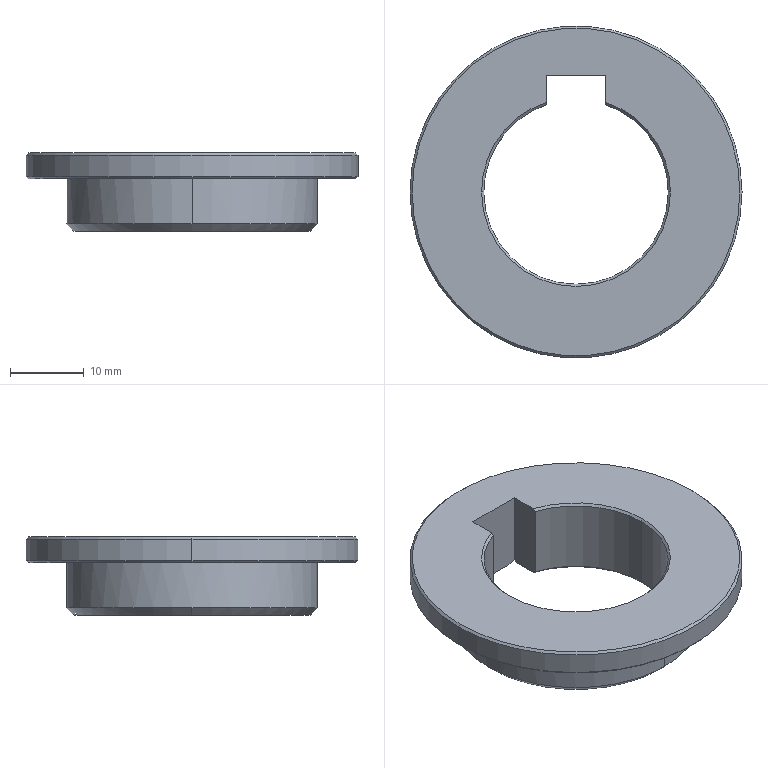Part | NX | 1 solid | 26 faces | box 45 x 45 x 10.6 mm | volume 6440 mm3 | cone 12 | plane 7 | cylinder 7 | commonest cylinder face diameters 25 x3 34 x2 45 x2
STEP:
#1=CARTESIAN_POINT('',(22.2,0.,-3.5));
#2=VERTEX_POINT('',#1);
#3=CARTESIAN_POINT('',(-22.2,0.,-3.5));
#4=VERTEX_POINT('',#3);
#5=CARTESIAN_POINT('',(0.,0.,-3.5));
#6=DIRECTION('',(0.,0.,1.));
#7=DIRECTION('',(1.,0.,0.));
#8=AXIS2_PLACEMENT_3D('',#5,#6,#7);
#9=CIRCLE('',#8,22.2);
#10=EDGE_CURVE('',#2,#4,#9,.T.);
#11=ORIENTED_EDGE('',*,*,#10,.F.);
#12=CARTESIAN_POINT('',(0.,0.,-3.5));
#13=DIRECTION('',(0.,0.,1.));
#14=DIRECTION('',(1.,0.,0.));
#15=AXIS2_PLACEMENT_3D('',#12,#13,#14);
#16=CIRCLE('',#15,22.2);
#17=EDGE_CURVE('',#4,#2,#16,.T.);
#18=ORIENTED_EDGE('',*,*,#17,.F.);
#19=EDGE_LOOP('',(#11,#18));
#20=FACE_BOUND('',#19,.T.);
#21=CARTESIAN_POINT('',(0.,-17.,-3.5));
#22=VERTEX_POINT('',#21);
#23=CARTESIAN_POINT('',(0.,17.,-3.5));
#24=VERTEX_POINT('',#23);
#25=CARTESIAN_POINT('',(0.,0.,-3.5));
#26=DIRECTION('',(0.,0.,1.));
#27=DIRECTION('',(0.,1.,0.));
#28=AXIS2_PLACEMENT_3D('',#25,#26,#27);
#29=CIRCLE('',#28,17.);
#30=EDGE_CURVE('',#22,#24,#29,.T.);
#31=ORIENTED_EDGE('',*,*,#30,.T.);
#32=CARTESIAN_POINT('',(0.,0.,-3.5));
#33=DIRECTION('',(0.,0.,1.));
#34=DIRECTION('',(0.,1.,0.));
#35=AXIS2_PLACEMENT_3D('',#32,#33,#34);
#36=CIRCLE('',#35,17.);
#37=EDGE_CURVE('',#24,#22,#36,.T.);
#38=ORIENTED_EDGE('',*,*,#37,.T.);
#39=EDGE_LOOP('',(#31,#38));
#40=FACE_BOUND('',#39,.T.);
#41=CARTESIAN_POINT('',(0.,0.,-3.5));
#42=DIRECTION('',(0.,0.,1.));
#43=DIRECTION('',(1.,0.,0.));
#44=AXIS2_PLACEMENT_3D('',#41,#42,#43);
#45=PLANE('',#44);
#46=ADVANCED_FACE('',(#20,#40),#45,.F.);
#47=CARTESIAN_POINT('',(22.5,0.,-3.2));
#48=VERTEX_POINT('',#47);
#49=CARTESIAN_POINT('',(-22.5,0.,-3.2));
#50=VERTEX_POINT('',#49);
#51=CARTESIAN_POINT('',(0.,0.,-3.2));
#52=DIRECTION('',(0.,0.,1.));
#53=DIRECTION('',(1.,0.,0.));
#54=AXIS2_PLACEMENT_3D('',#51,#52,#53);
#55=CIRCLE('',#54,22.5);
#56=EDGE_CURVE('',#48,#50,#55,.T.);
#57=ORIENTED_EDGE('',*,*,#56,.T.);
#58=CARTESIAN_POINT('',(-22.5,0.,-0.3));
#59=VERTEX_POINT('',#58);
#60=CARTESIAN_POINT('',(-22.5,0.,0.));
#61=DIRECTION('',(0.,0.,-1.));
#62=VECTOR('',#61,1000.);
#63=LINE('',#60,#62);
#64=EDGE_CURVE('',#50,#59,#63,.F.);
#65=ORIENTED_EDGE('',*,*,#64,.T.);
#66=CARTESIAN_POINT('',(22.5,0.,-0.3));
#67=VERTEX_POINT('',#66);
#68=CARTESIAN_POINT('',(0.,0.,-0.3));
#69=DIRECTION('',(0.,0.,-1.));
#70=DIRECTION('',(-1.,0.,0.));
#71=AXIS2_PLACEMENT_3D('',#68,#69,#70);
#72=CIRCLE('',#71,22.5);
#73=EDGE_CURVE('',#59,#67,#72,.T.);
#74=ORIENTED_EDGE('',*,*,#73,.T.);
#75=CARTESIAN_POINT('',(22.5,0.,0.));
#76=DIRECTION('',(0.,0.,-1.));
#77=VECTOR('',#76,1000.);
#78=LINE('',#75,#77);
#79=EDGE_CURVE('',#48,#67,#78,.F.);
#80=ORIENTED_EDGE('',*,*,#79,.F.);
#81=EDGE_LOOP('',(#57,#65,#74,#80));
#82=FACE_BOUND('',#81,.T.);
#83=CARTESIAN_POINT('',(0.,0.,0.));
#84=DIRECTION('',(0.,0.,-1.));
#85=DIRECTION('',(-1.,0.,0.));
#86=AXIS2_PLACEMENT_3D('',#83,#84,#85);
#87=CYLINDRICAL_SURFACE('',#86,22.5);
#88=ADVANCED_FACE('',(#82),#87,.T.);
#89=CARTESIAN_POINT('',(12.5,0.,-0.3));
#90=VERTEX_POINT('',#89);
#91=CARTESIAN_POINT('',(12.5,0.,-10.3));
#92=VERTEX_POINT('',#91);
#93=CARTESIAN_POINT('',(12.5,0.,0.));
#94=DIRECTION('',(0.,0.,-1.));
#95=VECTOR('',#94,1000.);
#96=LINE('',#93,#95);
#97=EDGE_CURVE('',#90,#92,#96,.T.);
#98=ORIENTED_EDGE('',*,*,#97,.F.);
#99=CARTESIAN_POINT('',(4.,11.843,-0.3));
#100=VERTEX_POINT('',#99);
#101=CARTESIAN_POINT('',(0.,0.,-0.3));
#102=DIRECTION('',(0.,0.,1.));
#103=DIRECTION('',(1.,0.,0.));
#104=AXIS2_PLACEMENT_3D('',#101,#102,#103);
#105=CIRCLE('',#104,12.5);
#106=EDGE_CURVE('',#90,#100,#105,.T.);
#107=ORIENTED_EDGE('',*,*,#106,.T.);
#108=CARTESIAN_POINT('',(4.,11.843,-10.3));
#109=VERTEX_POINT('',#108);
#110=CARTESIAN_POINT('',(4.,11.843,0.));
#111=DIRECTION('',(0.,0.,-1.));
#112=VECTOR('',#111,1000.);
#113=LINE('',#110,#112);
#114=EDGE_CURVE('',#100,#109,#113,.T.);
#115=ORIENTED_EDGE('',*,*,#114,.T.);
#116=CARTESIAN_POINT('',(0.,0.,-10.3));
#117=DIRECTION('',(0.,0.,-1.));
#118=DIRECTION('',(-1.,0.,0.));
#119=AXIS2_PLACEMENT_3D('',#116,#117,#118);
#120=CIRCLE('',#119,12.5);
#121=EDGE_CURVE('',#109,#92,#120,.T.);
#122=ORIENTED_EDGE('',*,*,#121,.T.);
#123=EDGE_LOOP('',(#98,#107,#115,#122));
#124=FACE_BOUND('',#123,.T.);
#125=CARTESIAN_POINT('',(0.,0.,0.));
#126=DIRECTION('',(0.,0.,-1.));
#127=DIRECTION('',(-1.,0.,0.));
#128=AXIS2_PLACEMENT_3D('',#125,#126,#127);
#129=CYLINDRICAL_SURFACE('',#128,12.5);
#130=ADVANCED_FACE('',(#124),#129,.F.);
#131=CARTESIAN_POINT('',(22.2,0.,0.));
#132=VERTEX_POINT('',#131);
#133=CARTESIAN_POINT('',(-22.2,0.,0.));
#134=VERTEX_POINT('',#133);
#135=CARTESIAN_POINT('',(0.,0.,0.));
#136=DIRECTION('',(0.,0.,-1.));
#137=DIRECTION('',(-1.,0.,0.));
#138=AXIS2_PLACEMENT_3D('',#135,#136,#137);
#139=CIRCLE('',#138,22.2);
#140=EDGE_CURVE('',#132,#134,#139,.T.);
#141=ORIENTED_EDGE('',*,*,#140,.F.);
#142=CARTESIAN_POINT('',(0.,0.,0.));
#143=DIRECTION('',(0.,0.,-1.));
#144=DIRECTION('',(-1.,0.,0.));
#145=AXIS2_PLACEMENT_3D('',#142,#143,#144);
#146=CIRCLE('',#145,22.2);
#147=EDGE_CURVE('',#134,#132,#146,.T.);
#148=ORIENTED_EDGE('',*,*,#147,.F.);
#149=EDGE_LOOP('',(#141,#148));
#150=FACE_BOUND('',#149,.T.);
#151=CARTESIAN_POINT('',(-4.,12.159,0.));
#152=VERTEX_POINT('',#151);
#153=CARTESIAN_POINT('',(-12.8,0.,0.));
#154=VERTEX_POINT('',#153);
#155=CARTESIAN_POINT('',(0.,0.,0.));
#156=DIRECTION('',(0.,0.,1.));
#157=DIRECTION('',(1.,0.,0.));
#158=AXIS2_PLACEMENT_3D('',#155,#156,#157);
#159=CIRCLE('',#158,12.8);
#160=EDGE_CURVE('',#152,#154,#159,.T.);
#161=ORIENTED_EDGE('',*,*,#160,.F.);
#162=CARTESIAN_POINT('',(-4.,15.8,0.));
#163=VERTEX_POINT('',#162);
#164=CARTESIAN_POINT('',(-4.,0.,0.));
#165=DIRECTION('',(0.,-1.,0.));
#166=VECTOR('',#165,1000.);
#167=LINE('',#164,#166);
#168=EDGE_CURVE('',#163,#152,#167,.T.);
#169=ORIENTED_EDGE('',*,*,#168,.F.);
#170=CARTESIAN_POINT('',(4.,15.8,0.));
#171=VERTEX_POINT('',#170);
#172=CARTESIAN_POINT('',(0.,15.8,0.));
#173=DIRECTION('',(-1.,0.,0.));
#174=VECTOR('',#173,1000.);
#175=LINE('',#172,#174);
#176=EDGE_CURVE('',#171,#163,#175,.T.);
#177=ORIENTED_EDGE('',*,*,#176,.F.);
#178=CARTESIAN_POINT('',(4.,12.159,0.));
#179=VERTEX_POINT('',#178);
#180=CARTESIAN_POINT('',(4.,0.,0.));
#181=DIRECTION('',(0.,1.,0.));
#182=VECTOR('',#181,1000.);
#183=LINE('',#180,#182);
#184=EDGE_CURVE('',#179,#171,#183,.T.);
#185=ORIENTED_EDGE('',*,*,#184,.F.);
#186=CARTESIAN_POINT('',(12.8,0.,0.));
#187=VERTEX_POINT('',#186);
#188=CARTESIAN_POINT('',(0.,0.,0.));
#189=DIRECTION('',(0.,0.,1.));
#190=DIRECTION('',(1.,0.,0.));
#191=AXIS2_PLACEMENT_3D('',#188,#189,#190);
#192=CIRCLE('',#191,12.8);
#193=EDGE_CURVE('',#187,#179,#192,.T.);
#194=ORIENTED_EDGE('',*,*,#193,.F.);
#195=CARTESIAN_POINT('',(0.,0.,0.));
#196=DIRECTION('',(0.,0.,1.));
#197=DIRECTION('',(1.,0.,0.));
#198=AXIS2_PLACEMENT_3D('',#195,#196,#197);
#199=CIRCLE('',#198,12.8);
#200=EDGE_CURVE('',#154,#187,#199,.T.);
#201=ORIENTED_EDGE('',*,*,#200,.F.);
#202=EDGE_LOOP('',(#161,#169,#177,#185,#194,#201));
#203=FACE_BOUND('',#202,.T.);
#204=CARTESIAN_POINT('',(0.,0.,0.));
#205=DIRECTION('',(0.,0.,1.));
#206=DIRECTION('',(1.,0.,0.));
#207=AXIS2_PLACEMENT_3D('',#204,#205,#206);
#208=PLANE('',#207);
#209=ADVANCED_FACE('',(#150,#203),#208,.T.);
#210=CARTESIAN_POINT('',(0.,17.,-9.6));
#211=VERTEX_POINT('',#210);
#212=CARTESIAN_POINT('',(17.,0.,-9.6));
#213=VERTEX_POINT('',#212);
#214=CARTESIAN_POINT('',(0.,0.,-9.6));
#215=DIRECTION('',(0.,0.,-1.));
#216=DIRECTION('',(1.,0.,0.));
#217=AXIS2_PLACEMENT_3D('',#214,#215,#216);
#218=CIRCLE('',#217,17.);
#219=EDGE_CURVE('',#211,#213,#218,.T.);
#220=ORIENTED_EDGE('',*,*,#219,.F.);
#221=CARTESIAN_POINT('',(0.,17.,-3.5));
#222=DIRECTION('',(0.,0.,-1.));
#223=VECTOR('',#222,1000.);
#224=LINE('',#221,#223);
#225=EDGE_CURVE('',#211,#24,#224,.F.);
#226=ORIENTED_EDGE('',*,*,#225,.T.);
#227=ORIENTED_EDGE('',*,*,#30,.F.);
#228=CARTESIAN_POINT('',(0.,-17.,-9.6));
#229=VERTEX_POINT('',#228);
#230=CARTESIAN_POINT('',(0.,-17.,-3.5));
#231=DIRECTION('',(0.,0.,-1.));
#232=VECTOR('',#231,1000.);
#233=LINE('',#230,#232);
#234=EDGE_CURVE('',#229,#22,#233,.F.);
#235=ORIENTED_EDGE('',*,*,#234,.F.);
#236=CARTESIAN_POINT('',(0.,0.,-9.6));
#237=DIRECTION('',(0.,0.,-1.));
#238=DIRECTION('',(1.,0.,0.));
#239=AXIS2_PLACEMENT_3D('',#236,#237,#238);
#240=CIRCLE('',#239,17.);
#241=EDGE_CURVE('',#213,#229,#240,.T.);
#242=ORIENTED_EDGE('',*,*,#241,.F.);
#243=EDGE_LOOP('',(#220,#226,#227,#235,#242));
#244=FACE_BOUND('',#243,.T.);
#245=CARTESIAN_POINT('',(0.,0.,-3.5));
#246=DIRECTION('',(0.,0.,-1.));
#247=DIRECTION('',(0.,1.,0.));
#248=AXIS2_PLACEMENT_3D('',#245,#246,#247);
#249=CYLINDRICAL_SURFACE('',#248,17.);
#250=ADVANCED_FACE('',(#244),#249,.T.);
#251=CARTESIAN_POINT('',(4.,12.159,-10.6));
#252=VERTEX_POINT('',#251);
#253=CARTESIAN_POINT('',(12.8,0.,-10.6));
#254=VERTEX_POINT('',#253);
#255=CARTESIAN_POINT('',(0.,0.,-10.6));
#256=DIRECTION('',(0.,0.,-1.));
#257=DIRECTION('',(-1.,0.,0.));
#258=AXIS2_PLACEMENT_3D('',#255,#256,#257);
#259=CIRCLE('',#258,12.8);
#260=EDGE_CURVE('',#252,#254,#259,.T.);
#261=ORIENTED_EDGE('',*,*,#260,.F.);
#262=CARTESIAN_POINT('',(4.,15.492,-10.6));
#263=VERTEX_POINT('',#262);
#264=CARTESIAN_POINT('',(4.,0.,-10.6));
#265=DIRECTION('',(0.,1.,0.));
#266=VECTOR('',#265,1000.);
#267=LINE('',#264,#266);
#268=EDGE_CURVE('',#252,#263,#267,.T.);
#269=ORIENTED_EDGE('',*,*,#268,.T.);
#270=CARTESIAN_POINT('',(16.,0.,-10.6));
#271=VERTEX_POINT('',#270);
#272=CARTESIAN_POINT('',(0.,0.,-10.6));
#273=DIRECTION('',(0.,0.,-1.));
#274=DIRECTION('',(1.,0.,0.));
#275=AXIS2_PLACEMENT_3D('',#272,#273,#274);
#276=CIRCLE('',#275,16.);
#277=EDGE_CURVE('',#263,#271,#276,.T.);
#278=ORIENTED_EDGE('',*,*,#277,.T.);
#279=CARTESIAN_POINT('',(-16.,0.,-10.6));
#280=VERTEX_POINT('',#279);
#281=CARTESIAN_POINT('',(0.,0.,-10.6));
#282=DIRECTION('',(0.,0.,-1.));
#283=DIRECTION('',(1.,0.,0.));
#284=AXIS2_PLACEMENT_3D('',#281,#282,#283);
#285=CIRCLE('',#284,16.);
#286=EDGE_CURVE('',#271,#280,#285,.T.);
#287=ORIENTED_EDGE('',*,*,#286,.T.);
#288=CARTESIAN_POINT('',(-4.,15.492,-10.6));
#289=VERTEX_POINT('',#288);
#290=CARTESIAN_POINT('',(0.,0.,-10.6));
#291=DIRECTION('',(0.,0.,-1.));
#292=DIRECTION('',(1.,0.,0.));
#293=AXIS2_PLACEMENT_3D('',#290,#291,#292);
#294=CIRCLE('',#293,16.);
#295=EDGE_CURVE('',#280,#289,#294,.T.);
#296=ORIENTED_EDGE('',*,*,#295,.T.);
#297=CARTESIAN_POINT('',(-4.,12.159,-10.6));
#298=VERTEX_POINT('',#297);
#299=CARTESIAN_POINT('',(-4.,0.,-10.6));
#300=DIRECTION('',(0.,-1.,0.));
#301=VECTOR('',#300,1000.);
#302=LINE('',#299,#301);
#303=EDGE_CURVE('',#289,#298,#302,.T.);
#304=ORIENTED_EDGE('',*,*,#303,.T.);
#305=CARTESIAN_POINT('',(-12.8,0.,-10.6));
#306=VERTEX_POINT('',#305);
#307=CARTESIAN_POINT('',(0.,0.,-10.6));
#308=DIRECTION('',(0.,0.,-1.));
#309=DIRECTION('',(-1.,0.,0.));
#310=AXIS2_PLACEMENT_3D('',#307,#308,#309);
#311=CIRCLE('',#310,12.8);
#312=EDGE_CURVE('',#306,#298,#311,.T.);
#313=ORIENTED_EDGE('',*,*,#312,.F.);
#314=CARTESIAN_POINT('',(0.,0.,-10.6));
#315=DIRECTION('',(0.,0.,-1.));
#316=DIRECTION('',(-1.,0.,0.));
#317=AXIS2_PLACEMENT_3D('',#314,#315,#316);
#318=CIRCLE('',#317,12.8);
#319=EDGE_CURVE('',#254,#306,#318,.T.);
#320=ORIENTED_EDGE('',*,*,#319,.F.);
#321=EDGE_LOOP('',(#261,#269,#278,#287,#296,#304,#313,#320));
#322=FACE_BOUND('',#321,.T.);
#323=CARTESIAN_POINT('',(-14.369,9.107,-10.6));
#324=DIRECTION('',(0.,0.,1.));
#325=DIRECTION('',(1.,0.,0.));
#326=AXIS2_PLACEMENT_3D('',#323,#324,#325);
#327=PLANE('',#326);
#328=ADVANCED_FACE('',(#322),#327,.F.);
#329=ORIENTED_EDGE('',*,*,#219,.T.);
#330=CARTESIAN_POINT('',(16.,0.,-10.6));
#331=DIRECTION('',(0.7071,0.,0.7071));
#332=VECTOR('',#331,1000.);
#333=LINE('',#330,#332);
#334=EDGE_CURVE('',#213,#271,#333,.F.);
#335=ORIENTED_EDGE('',*,*,#334,.T.);
#336=ORIENTED_EDGE('',*,*,#277,.F.);
#337=CARTESIAN_POINT('',(4.,15.8,-10.302));
#338=VERTEX_POINT('',#337);
#339=CARTESIAN_POINT('',(4.,15.492,-10.6));
#340=CARTESIAN_POINT('',(4.,15.518,-10.575));
#341=CARTESIAN_POINT('',(4.,15.543,-10.55));
#342=CARTESIAN_POINT('',(4.,15.569,-10.525));
#343=CARTESIAN_POINT('',(4.,15.595,-10.501));
#344=CARTESIAN_POINT('',(4.,15.62,-10.476));
#345=CARTESIAN_POINT('',(4.,15.646,-10.451));
#346=CARTESIAN_POINT('',(4.,15.672,-10.426));
#347=CARTESIAN_POINT('',(4.,15.697,-10.401));
#348=CARTESIAN_POINT('',(4.,15.723,-10.376));
#349=CARTESIAN_POINT('',(4.,15.749,-10.351));
#350=CARTESIAN_POINT('',(4.,15.774,-10.326));
#351=CARTESIAN_POINT('',(4.,15.8,-10.302));
#352=B_SPLINE_CURVE_WITH_KNOTS('',3,(#339,#340,#341,#342,#343,#344,#345,#346,#347,#348,#349,#350,#351),.UNSPECIFIED.,.F.,.F.,(4,3,3,3,4),(0.,0.1072,0.2145,0.3217,0.4289),.UNSPECIFIED.);
#353=EDGE_CURVE('',#263,#338,#352,.T.);
#354=ORIENTED_EDGE('',*,*,#353,.T.);
#355=CARTESIAN_POINT('',(2.522,15.8,-10.6));
#356=VERTEX_POINT('',#355);
#357=CARTESIAN_POINT('',(4.,15.8,-10.302));
#358=CARTESIAN_POINT('',(3.878,15.8,-10.331));
#359=CARTESIAN_POINT('',(3.756,15.8,-10.36));
#360=CARTESIAN_POINT('',(3.634,15.8,-10.388));
#361=CARTESIAN_POINT('',(3.511,15.8,-10.415));
#362=CARTESIAN_POINT('',(3.389,15.8,-10.441));
#363=CARTESIAN_POINT('',(3.265,15.8,-10.466));
#364=CARTESIAN_POINT('',(3.142,15.8,-10.491));
#365=CARTESIAN_POINT('',(3.019,15.8,-10.515));
#366=CARTESIAN_POINT('',(2.895,15.8,-10.537));
#367=CARTESIAN_POINT('',(2.771,15.8,-10.559));
#368=CARTESIAN_POINT('',(2.646,15.8,-10.58));
#369=CARTESIAN_POINT('',(2.522,15.8,-10.6));
#370=B_SPLINE_CURVE_WITH_KNOTS('',3,(#357,#358,#359,#360,#361,#362,#363,#364,#365,#366,#367,#368,#369),.UNSPECIFIED.,.F.,.F.,(4,3,3,3,4),(0.,0.3761,0.7528,1.13,1.508),.UNSPECIFIED.);
#371=EDGE_CURVE('',#338,#356,#370,.T.);
#372=ORIENTED_EDGE('',*,*,#371,.T.);
#373=CARTESIAN_POINT('',(-2.522,15.8,-10.6));
#374=VERTEX_POINT('',#373);
#375=CARTESIAN_POINT('',(0.,0.,-10.6));
#376=DIRECTION('',(0.,0.,-1.));
#377=DIRECTION('',(1.,0.,0.));
#378=AXIS2_PLACEMENT_3D('',#375,#376,#377);
#379=CIRCLE('',#378,16.);
#380=EDGE_CURVE('',#374,#356,#379,.T.);
#381=ORIENTED_EDGE('',*,*,#380,.F.);
#382=CARTESIAN_POINT('',(-4.,15.8,-10.302));
#383=VERTEX_POINT('',#382);
#384=CARTESIAN_POINT('',(-2.522,15.8,-10.6));
#385=CARTESIAN_POINT('',(-2.646,15.8,-10.58));
#386=CARTESIAN_POINT('',(-2.77,15.8,-10.56));
#387=CARTESIAN_POINT('',(-2.893,15.8,-10.537));
#388=CARTESIAN_POINT('',(-3.017,15.8,-10.515));
#389=CARTESIAN_POINT('',(-3.14,15.8,-10.491));
#390=CARTESIAN_POINT('',(-3.264,15.8,-10.466));
#391=CARTESIAN_POINT('',(-3.387,15.8,-10.442));
#392=CARTESIAN_POINT('',(-3.51,15.8,-10.415));
#393=CARTESIAN_POINT('',(-3.633,15.8,-10.388));
#394=CARTESIAN_POINT('',(-3.755,15.8,-10.36));
#395=CARTESIAN_POINT('',(-3.878,15.8,-10.332));
#396=CARTESIAN_POINT('',(-4.,15.8,-10.302));
#397=B_SPLINE_CURVE_WITH_KNOTS('',3,(#384,#385,#386,#387,#388,#389,#390,#391,#392,#393,#394,#395,#396),.UNSPECIFIED.,.F.,.F.,(4,3,3,3,4),(0.,0.3767,0.7537,1.131,1.508),.UNSPECIFIED.);
#398=EDGE_CURVE('',#374,#383,#397,.T.);
#399=ORIENTED_EDGE('',*,*,#398,.T.);
#400=CARTESIAN_POINT('',(-4.,15.8,-10.302));
#401=CARTESIAN_POINT('',(-4.,15.774,-10.326));
#402=CARTESIAN_POINT('',(-4.,15.749,-10.351));
#403=CARTESIAN_POINT('',(-4.,15.723,-10.376));
#404=CARTESIAN_POINT('',(-4.,15.697,-10.401));
#405=CARTESIAN_POINT('',(-4.,15.672,-10.426));
#406=CARTESIAN_POINT('',(-4.,15.646,-10.451));
#407=CARTESIAN_POINT('',(-4.,15.62,-10.476));
#408=CARTESIAN_POINT('',(-4.,15.595,-10.501));
#409=CARTESIAN_POINT('',(-4.,15.569,-10.525));
#410=CARTESIAN_POINT('',(-4.,15.543,-10.55));
#411=CARTESIAN_POINT('',(-4.,15.518,-10.575));
#412=CARTESIAN_POINT('',(-4.,15.492,-10.6));
#413=B_SPLINE_CURVE_WITH_KNOTS('',3,(#400,#401,#402,#403,#404,#405,#406,#407,#408,#409,#410,#411,#412),.UNSPECIFIED.,.F.,.F.,(4,3,3,3,4),(0.,0.1072,0.2145,0.3217,0.4289),.UNSPECIFIED.);
#414=EDGE_CURVE('',#383,#289,#413,.T.);
#415=ORIENTED_EDGE('',*,*,#414,.T.);
#416=ORIENTED_EDGE('',*,*,#295,.F.);
#417=CARTESIAN_POINT('',(-17.,0.,-9.6));
#418=VERTEX_POINT('',#417);
#419=CARTESIAN_POINT('',(-16.,0.,-10.6));
#420=DIRECTION('',(-0.7071,0.,0.7071));
#421=VECTOR('',#420,1000.);
#422=LINE('',#419,#421);
#423=EDGE_CURVE('',#418,#280,#422,.F.);
#424=ORIENTED_EDGE('',*,*,#423,.F.);
#425=CARTESIAN_POINT('',(0.,0.,-9.6));
#426=DIRECTION('',(0.,0.,-1.));
#427=DIRECTION('',(1.,0.,0.));
#428=AXIS2_PLACEMENT_3D('',#425,#426,#427);
#429=CIRCLE('',#428,17.);
#430=EDGE_CURVE('',#418,#211,#429,.T.);
#431=ORIENTED_EDGE('',*,*,#430,.T.);
#432=EDGE_LOOP('',(#329,#335,#336,#354,#372,#381,#399,#415,#416,#424,#431));
#433=FACE_BOUND('',#432,.T.);
#434=CARTESIAN_POINT('',(0.,0.,-10.6));
#435=DIRECTION('',(0.,0.,1.));
#436=DIRECTION('',(1.,0.,0.));
#437=AXIS2_PLACEMENT_3D('',#434,#435,#436);
#438=CONICAL_SURFACE('',#437,16.,0.7854);
#439=ADVANCED_FACE('',(#433),#438,.T.);
#440=ORIENTED_EDGE('',*,*,#380,.T.);
#441=CARTESIAN_POINT('',(0.,15.8,-10.6));
#442=DIRECTION('',(-1.,0.,0.));
#443=VECTOR('',#442,1000.);
#444=LINE('',#441,#443);
#445=EDGE_CURVE('',#356,#374,#444,.T.);
#446=ORIENTED_EDGE('',*,*,#445,.T.);
#447=EDGE_LOOP('',(#440,#446));
#448=FACE_BOUND('',#447,.T.);
#449=CARTESIAN_POINT('',(-14.369,9.107,-10.6));
#450=DIRECTION('',(0.,0.,1.));
#451=DIRECTION('',(1.,0.,0.));
#452=AXIS2_PLACEMENT_3D('',#449,#450,#451);
#453=PLANE('',#452);
#454=ADVANCED_FACE('',(#448),#453,.F.);
#455=CARTESIAN_POINT('',(4.,15.8,-11.66));
#456=DIRECTION('',(0.,0.,1.));
#457=VECTOR('',#456,1000.);
#458=LINE('',#455,#457);
#459=EDGE_CURVE('',#338,#171,#458,.T.);
#460=ORIENTED_EDGE('',*,*,#459,.T.);
#461=ORIENTED_EDGE('',*,*,#176,.T.);
#462=CARTESIAN_POINT('',(-4.,15.8,-11.66));
#463=DIRECTION('',(0.,0.,1.));
#464=VECTOR('',#463,1000.);
#465=LINE('',#462,#464);
#466=EDGE_CURVE('',#383,#163,#465,.T.);
#467=ORIENTED_EDGE('',*,*,#466,.F.);
#468=ORIENTED_EDGE('',*,*,#398,.F.);
#469=ORIENTED_EDGE('',*,*,#445,.F.);
#470=ORIENTED_EDGE('',*,*,#371,.F.);
#471=EDGE_LOOP('',(#460,#461,#467,#468,#469,#470));
#472=FACE_BOUND('',#471,.T.);
#473=CARTESIAN_POINT('',(4.,15.8,-11.66));
#474=DIRECTION('',(0.,-1.,0.));
#475=DIRECTION('',(0.,0.,-1.));
#476=AXIS2_PLACEMENT_3D('',#473,#474,#475);
#477=PLANE('',#476);
#478=ADVANCED_FACE('',(#472),#477,.T.);
#479=CARTESIAN_POINT('',(-4.,11.843,-0.3));
#480=VERTEX_POINT('',#479);
#481=CARTESIAN_POINT('',(-4.,11.843,-10.3));
#482=VERTEX_POINT('',#481);
#483=CARTESIAN_POINT('',(-4.,11.843,0.));
#484=DIRECTION('',(0.,0.,-1.));
#485=VECTOR('',#484,1000.);
#486=LINE('',#483,#485);
#487=EDGE_CURVE('',#480,#482,#486,.T.);
#488=ORIENTED_EDGE('',*,*,#487,.T.);
#489=CARTESIAN_POINT('',(-4.,11.843,-10.3));
#490=CARTESIAN_POINT('',(-4.,11.869,-10.325));
#491=CARTESIAN_POINT('',(-4.,11.895,-10.35));
#492=CARTESIAN_POINT('',(-4.,11.922,-10.375));
#493=CARTESIAN_POINT('',(-4.,11.948,-10.4));
#494=CARTESIAN_POINT('',(-4.,11.975,-10.425));
#495=CARTESIAN_POINT('',(-4.,12.001,-10.45));
#496=CARTESIAN_POINT('',(-4.,12.027,-10.475));
#497=CARTESIAN_POINT('',(-4.,12.054,-10.5));
#498=CARTESIAN_POINT('',(-4.,12.08,-10.525));
#499=CARTESIAN_POINT('',(-4.,12.106,-10.55));
#500=CARTESIAN_POINT('',(-4.,12.133,-10.575));
#501=CARTESIAN_POINT('',(-4.,12.159,-10.6));
#502=B_SPLINE_CURVE_WITH_KNOTS('',3,(#489,#490,#491,#492,#493,#494,#495,#496,#497,#498,#499,#500,#501),.UNSPECIFIED.,.F.,.F.,(4,3,3,3,4),(0.,0.109,0.2179,0.3269,0.4359),.UNSPECIFIED.);
#503=EDGE_CURVE('',#482,#298,#502,.T.);
#504=ORIENTED_EDGE('',*,*,#503,.T.);
#505=ORIENTED_EDGE('',*,*,#303,.F.);
#506=ORIENTED_EDGE('',*,*,#414,.F.);
#507=ORIENTED_EDGE('',*,*,#466,.T.);
#508=ORIENTED_EDGE('',*,*,#168,.T.);
#509=CARTESIAN_POINT('',(-4.,12.159,0.));
#510=CARTESIAN_POINT('',(-4.,12.133,-0.02502));
#511=CARTESIAN_POINT('',(-4.,12.106,-0.05003));
#512=CARTESIAN_POINT('',(-4.,12.08,-0.07504));
#513=CARTESIAN_POINT('',(-4.,12.054,-0.1));
#514=CARTESIAN_POINT('',(-4.,12.027,-0.1251));
#515=CARTESIAN_POINT('',(-4.,12.001,-0.1501));
#516=CARTESIAN_POINT('',(-4.,11.975,-0.1751));
#517=CARTESIAN_POINT('',(-4.,11.948,-0.2));
#518=CARTESIAN_POINT('',(-4.,11.922,-0.225));
#519=CARTESIAN_POINT('',(-4.,11.895,-0.25));
#520=CARTESIAN_POINT('',(-4.,11.869,-0.275));
#521=CARTESIAN_POINT('',(-4.,11.843,-0.3));
#522=B_SPLINE_CURVE_WITH_KNOTS('',3,(#509,#510,#511,#512,#513,#514,#515,#516,#517,#518,#519,#520,#521),.UNSPECIFIED.,.F.,.F.,(4,3,3,3,4),(0.,0.109,0.2179,0.3269,0.4359),.UNSPECIFIED.);
#523=EDGE_CURVE('',#152,#480,#522,.T.);
#524=ORIENTED_EDGE('',*,*,#523,.T.);
#525=EDGE_LOOP('',(#488,#504,#505,#506,#507,#508,#524));
#526=FACE_BOUND('',#525,.T.);
#527=CARTESIAN_POINT('',(-4.,15.8,-11.66));
#528=DIRECTION('',(1.,0.,0.));
#529=DIRECTION('',(0.,1.,0.));
#530=AXIS2_PLACEMENT_3D('',#527,#528,#529);
#531=PLANE('',#530);
#532=ADVANCED_FACE('',(#526),#531,.T.);
#533=ORIENTED_EDGE('',*,*,#114,.F.);
#534=CARTESIAN_POINT('',(4.,11.843,-0.3));
#535=CARTESIAN_POINT('',(4.,11.869,-0.275));
#536=CARTESIAN_POINT('',(4.,11.895,-0.25));
#537=CARTESIAN_POINT('',(4.,11.922,-0.225));
#538=CARTESIAN_POINT('',(4.,11.948,-0.2));
#539=CARTESIAN_POINT('',(4.,11.975,-0.1751));
#540=CARTESIAN_POINT('',(4.,12.001,-0.1501));
#541=CARTESIAN_POINT('',(4.,12.027,-0.1251));
#542=CARTESIAN_POINT('',(4.,12.054,-0.1));
#543=CARTESIAN_POINT('',(4.,12.08,-0.07504));
#544=CARTESIAN_POINT('',(4.,12.106,-0.05003));
#545=CARTESIAN_POINT('',(4.,12.133,-0.02502));
#546=CARTESIAN_POINT('',(4.,12.159,0.));
#547=B_SPLINE_CURVE_WITH_KNOTS('',3,(#534,#535,#536,#537,#538,#539,#540,#541,#542,#543,#544,#545,#546),.UNSPECIFIED.,.F.,.F.,(4,3,3,3,4),(0.,0.109,0.2179,0.3269,0.4359),.UNSPECIFIED.);
#548=EDGE_CURVE('',#100,#179,#547,.T.);
#549=ORIENTED_EDGE('',*,*,#548,.T.);
#550=ORIENTED_EDGE('',*,*,#184,.T.);
#551=ORIENTED_EDGE('',*,*,#459,.F.);
#552=ORIENTED_EDGE('',*,*,#353,.F.);
#553=ORIENTED_EDGE('',*,*,#268,.F.);
#554=CARTESIAN_POINT('',(4.,12.159,-10.6));
#555=CARTESIAN_POINT('',(4.,12.133,-10.575));
#556=CARTESIAN_POINT('',(4.,12.106,-10.55));
#557=CARTESIAN_POINT('',(4.,12.08,-10.525));
#558=CARTESIAN_POINT('',(4.,12.054,-10.5));
#559=CARTESIAN_POINT('',(4.,12.027,-10.475));
#560=CARTESIAN_POINT('',(4.,12.001,-10.45));
#561=CARTESIAN_POINT('',(4.,11.975,-10.425));
#562=CARTESIAN_POINT('',(4.,11.948,-10.4));
#563=CARTESIAN_POINT('',(4.,11.922,-10.375));
#564=CARTESIAN_POINT('',(4.,11.895,-10.35));
#565=CARTESIAN_POINT('',(4.,11.869,-10.325));
#566=CARTESIAN_POINT('',(4.,11.843,-10.3));
#567=B_SPLINE_CURVE_WITH_KNOTS('',3,(#554,#555,#556,#557,#558,#559,#560,#561,#562,#563,#564,#565,#566),.UNSPECIFIED.,.F.,.F.,(4,3,3,3,4),(0.,0.109,0.2179,0.3269,0.4359),.UNSPECIFIED.);
#568=EDGE_CURVE('',#252,#109,#567,.T.);
#569=ORIENTED_EDGE('',*,*,#568,.T.);
#570=EDGE_LOOP('',(#533,#549,#550,#551,#552,#553,#569));
#571=FACE_BOUND('',#570,.T.);
#572=CARTESIAN_POINT('',(4.,11.843,-11.66));
#573=DIRECTION('',(-1.,0.,0.));
#574=DIRECTION('',(0.,0.,1.));
#575=AXIS2_PLACEMENT_3D('',#572,#573,#574);
#576=PLANE('',#575);
#577=ADVANCED_FACE('',(#571),#576,.T.);
#578=ORIENTED_EDGE('',*,*,#73,.F.);
#579=CARTESIAN_POINT('',(-22.2,0.,0.));
#580=DIRECTION('',(-0.7071,0.,-0.7071));
#581=VECTOR('',#580,1000.);
#582=LINE('',#579,#581);
#583=EDGE_CURVE('',#59,#134,#582,.F.);
#584=ORIENTED_EDGE('',*,*,#583,.T.);
#585=ORIENTED_EDGE('',*,*,#147,.T.);
#586=CARTESIAN_POINT('',(22.2,0.,0.));
#587=DIRECTION('',(0.7071,0.,-0.7071));
#588=VECTOR('',#587,1000.);
#589=LINE('',#586,#588);
#590=EDGE_CURVE('',#67,#132,#589,.F.);
#591=ORIENTED_EDGE('',*,*,#590,.F.);
#592=EDGE_LOOP('',(#578,#584,#585,#591));
#593=FACE_BOUND('',#592,.T.);
#594=CARTESIAN_POINT('',(0.,0.,0.));
#595=DIRECTION('',(0.,0.,-1.));
#596=DIRECTION('',(-1.,0.,0.));
#597=AXIS2_PLACEMENT_3D('',#594,#595,#596);
#598=CONICAL_SURFACE('',#597,22.2,0.7854);
#599=ADVANCED_FACE('',(#593),#598,.T.);
#600=CARTESIAN_POINT('',(-12.5,0.,-0.3));
#601=VERTEX_POINT('',#600);
#602=CARTESIAN_POINT('',(-12.8,0.,0.));
#603=DIRECTION('',(-0.7071,0.,0.7071));
#604=VECTOR('',#603,1000.);
#605=LINE('',#602,#604);
#606=EDGE_CURVE('',#601,#154,#605,.T.);
#607=ORIENTED_EDGE('',*,*,#606,.F.);
#608=CARTESIAN_POINT('',(0.,0.,-0.3));
#609=DIRECTION('',(0.,0.,1.));
#610=DIRECTION('',(1.,0.,0.));
#611=AXIS2_PLACEMENT_3D('',#608,#609,#610);
#612=CIRCLE('',#611,12.5);
#613=EDGE_CURVE('',#480,#601,#612,.T.);
#614=ORIENTED_EDGE('',*,*,#613,.F.);
#615=ORIENTED_EDGE('',*,*,#523,.F.);
#616=ORIENTED_EDGE('',*,*,#160,.T.);
#617=EDGE_LOOP('',(#607,#614,#615,#616));
#618=FACE_BOUND('',#617,.T.);
#619=CARTESIAN_POINT('',(0.,0.,0.));
#620=DIRECTION('',(0.,0.,1.));
#621=DIRECTION('',(1.,0.,0.));
#622=AXIS2_PLACEMENT_3D('',#619,#620,#621);
#623=CONICAL_SURFACE('',#622,12.8,0.7854);
#624=ADVANCED_FACE('',(#618),#623,.F.);
#625=ORIENTED_EDGE('',*,*,#56,.F.);
#626=CARTESIAN_POINT('',(22.2,0.,-3.5));
#627=DIRECTION('',(0.7071,0.,0.7071));
#628=VECTOR('',#627,1000.);
#629=LINE('',#626,#628);
#630=EDGE_CURVE('',#2,#48,#629,.T.);
#631=ORIENTED_EDGE('',*,*,#630,.F.);
#632=ORIENTED_EDGE('',*,*,#10,.T.);
#633=CARTESIAN_POINT('',(-22.2,0.,-3.5));
#634=DIRECTION('',(-0.7071,0.,0.7071));
#635=VECTOR('',#634,1000.);
#636=LINE('',#633,#635);
#637=EDGE_CURVE('',#4,#50,#636,.T.);
#638=ORIENTED_EDGE('',*,*,#637,.T.);
#639=EDGE_LOOP('',(#625,#631,#632,#638));
#640=FACE_BOUND('',#639,.T.);
#641=CARTESIAN_POINT('',(0.,0.,-3.5));
#642=DIRECTION('',(0.,0.,1.));
#643=DIRECTION('',(1.,0.,0.));
#644=AXIS2_PLACEMENT_3D('',#641,#642,#643);
#645=CONICAL_SURFACE('',#644,22.2,0.7854);
#646=ADVANCED_FACE('',(#640),#645,.T.);
#647=CARTESIAN_POINT('',(12.8,0.,-10.6));
#648=DIRECTION('',(0.7071,0.,-0.7071));
#649=VECTOR('',#648,1000.);
#650=LINE('',#647,#649);
#651=EDGE_CURVE('',#92,#254,#650,.T.);
#652=ORIENTED_EDGE('',*,*,#651,.F.);
#653=ORIENTED_EDGE('',*,*,#121,.F.);
#654=ORIENTED_EDGE('',*,*,#568,.F.);
#655=ORIENTED_EDGE('',*,*,#260,.T.);
#656=EDGE_LOOP('',(#652,#653,#654,#655));
#657=FACE_BOUND('',#656,.T.);
#658=CARTESIAN_POINT('',(0.,0.,-10.6));
#659=DIRECTION('',(0.,0.,-1.));
#660=DIRECTION('',(-1.,0.,0.));
#661=AXIS2_PLACEMENT_3D('',#658,#659,#660);
#662=CONICAL_SURFACE('',#661,12.8,0.7854);
#663=ADVANCED_FACE('',(#657),#662,.F.);
#664=ORIENTED_EDGE('',*,*,#64,.F.);
#665=CARTESIAN_POINT('',(0.,0.,-3.2));
#666=DIRECTION('',(0.,0.,1.));
#667=DIRECTION('',(1.,0.,0.));
#668=AXIS2_PLACEMENT_3D('',#665,#666,#667);
#669=CIRCLE('',#668,22.5);
#670=EDGE_CURVE('',#50,#48,#669,.T.);
#671=ORIENTED_EDGE('',*,*,#670,.T.);
#672=ORIENTED_EDGE('',*,*,#79,.T.);
#673=CARTESIAN_POINT('',(0.,0.,-0.3));
#674=DIRECTION('',(0.,0.,-1.));
#675=DIRECTION('',(-1.,0.,0.));
#676=AXIS2_PLACEMENT_3D('',#673,#674,#675);
#677=CIRCLE('',#676,22.5);
#678=EDGE_CURVE('',#67,#59,#677,.T.);
#679=ORIENTED_EDGE('',*,*,#678,.T.);
#680=EDGE_LOOP('',(#664,#671,#672,#679));
#681=FACE_BOUND('',#680,.T.);
#682=CARTESIAN_POINT('',(0.,0.,0.));
#683=DIRECTION('',(0.,0.,-1.));
#684=DIRECTION('',(-1.,0.,0.));
#685=AXIS2_PLACEMENT_3D('',#682,#683,#684);
#686=CYLINDRICAL_SURFACE('',#685,22.5);
#687=ADVANCED_FACE('',(#681),#686,.T.);
#688=ORIENTED_EDGE('',*,*,#630,.T.);
#689=ORIENTED_EDGE('',*,*,#670,.F.);
#690=ORIENTED_EDGE('',*,*,#637,.F.);
#691=ORIENTED_EDGE('',*,*,#17,.T.);
#692=EDGE_LOOP('',(#688,#689,#690,#691));
#693=FACE_BOUND('',#692,.T.);
#694=CARTESIAN_POINT('',(0.,0.,-3.5));
#695=DIRECTION('',(0.,0.,1.));
#696=DIRECTION('',(1.,0.,0.));
#697=AXIS2_PLACEMENT_3D('',#694,#695,#696);
#698=CONICAL_SURFACE('',#697,22.2,0.7854);
#699=ADVANCED_FACE('',(#693),#698,.T.);
#700=ORIENTED_EDGE('',*,*,#234,.T.);
#701=ORIENTED_EDGE('',*,*,#37,.F.);
#702=ORIENTED_EDGE('',*,*,#225,.F.);
#703=ORIENTED_EDGE('',*,*,#430,.F.);
#704=CARTESIAN_POINT('',(0.,0.,-9.6));
#705=DIRECTION('',(0.,0.,-1.));
#706=DIRECTION('',(1.,0.,0.));
#707=AXIS2_PLACEMENT_3D('',#704,#705,#706);
#708=CIRCLE('',#707,17.);
#709=EDGE_CURVE('',#229,#418,#708,.T.);
#710=ORIENTED_EDGE('',*,*,#709,.F.);
#711=EDGE_LOOP('',(#700,#701,#702,#703,#710));
#712=FACE_BOUND('',#711,.T.);
#713=CARTESIAN_POINT('',(0.,0.,-3.5));
#714=DIRECTION('',(0.,0.,-1.));
#715=DIRECTION('',(0.,1.,0.));
#716=AXIS2_PLACEMENT_3D('',#713,#714,#715);
#717=CYLINDRICAL_SURFACE('',#716,17.);
#718=ADVANCED_FACE('',(#712),#717,.T.);
#719=ORIENTED_EDGE('',*,*,#423,.T.);
#720=ORIENTED_EDGE('',*,*,#286,.F.);
#721=ORIENTED_EDGE('',*,*,#334,.F.);
#722=ORIENTED_EDGE('',*,*,#241,.T.);
#723=ORIENTED_EDGE('',*,*,#709,.T.);
#724=EDGE_LOOP('',(#719,#720,#721,#722,#723));
#725=FACE_BOUND('',#724,.T.);
#726=CARTESIAN_POINT('',(0.,0.,-10.6));
#727=DIRECTION('',(0.,0.,1.));
#728=DIRECTION('',(1.,0.,0.));
#729=AXIS2_PLACEMENT_3D('',#726,#727,#728);
#730=CONICAL_SURFACE('',#729,16.,0.7854);
#731=ADVANCED_FACE('',(#725),#730,.T.);
#732=ORIENTED_EDGE('',*,*,#140,.T.);
#733=ORIENTED_EDGE('',*,*,#583,.F.);
#734=ORIENTED_EDGE('',*,*,#678,.F.);
#735=ORIENTED_EDGE('',*,*,#590,.T.);
#736=EDGE_LOOP('',(#732,#733,#734,#735));
#737=FACE_BOUND('',#736,.T.);
#738=CARTESIAN_POINT('',(0.,0.,0.));
#739=DIRECTION('',(0.,0.,-1.));
#740=DIRECTION('',(-1.,0.,0.));
#741=AXIS2_PLACEMENT_3D('',#738,#739,#740);
#742=CONICAL_SURFACE('',#741,22.2,0.7854);
#743=ADVANCED_FACE('',(#737),#742,.T.);
#744=CARTESIAN_POINT('',(-12.5,0.,-10.3));
#745=VERTEX_POINT('',#744);
#746=CARTESIAN_POINT('',(0.,0.,-10.3));
#747=DIRECTION('',(0.,0.,-1.));
#748=DIRECTION('',(-1.,0.,0.));
#749=AXIS2_PLACEMENT_3D('',#746,#747,#748);
#750=CIRCLE('',#749,12.5);
#751=EDGE_CURVE('',#745,#482,#750,.T.);
#752=ORIENTED_EDGE('',*,*,#751,.F.);
#753=CARTESIAN_POINT('',(-12.8,0.,-10.6));
#754=DIRECTION('',(-0.7071,0.,-0.7071));
#755=VECTOR('',#754,1000.);
#756=LINE('',#753,#755);
#757=EDGE_CURVE('',#745,#306,#756,.T.);
#758=ORIENTED_EDGE('',*,*,#757,.T.);
#759=ORIENTED_EDGE('',*,*,#312,.T.);
#760=ORIENTED_EDGE('',*,*,#503,.F.);
#761=EDGE_LOOP('',(#752,#758,#759,#760));
#762=FACE_BOUND('',#761,.T.);
#763=CARTESIAN_POINT('',(0.,0.,-10.6));
#764=DIRECTION('',(0.,0.,-1.));
#765=DIRECTION('',(-1.,0.,0.));
#766=AXIS2_PLACEMENT_3D('',#763,#764,#765);
#767=CONICAL_SURFACE('',#766,12.8,0.7854);
#768=ADVANCED_FACE('',(#762),#767,.F.);
#769=CARTESIAN_POINT('',(0.,0.,-10.3));
#770=DIRECTION('',(0.,0.,-1.));
#771=DIRECTION('',(-1.,0.,0.));
#772=AXIS2_PLACEMENT_3D('',#769,#770,#771);
#773=CIRCLE('',#772,12.5);
#774=EDGE_CURVE('',#92,#745,#773,.T.);
#775=ORIENTED_EDGE('',*,*,#774,.F.);
#776=ORIENTED_EDGE('',*,*,#651,.T.);
#777=ORIENTED_EDGE('',*,*,#319,.T.);
#778=ORIENTED_EDGE('',*,*,#757,.F.);
#779=EDGE_LOOP('',(#775,#776,#777,#778));
#780=FACE_BOUND('',#779,.T.);
#781=CARTESIAN_POINT('',(0.,0.,-10.6));
#782=DIRECTION('',(0.,0.,-1.));
#783=DIRECTION('',(-1.,0.,0.));
#784=AXIS2_PLACEMENT_3D('',#781,#782,#783);
#785=CONICAL_SURFACE('',#784,12.8,0.7854);
#786=ADVANCED_FACE('',(#780),#785,.F.);
#787=ORIENTED_EDGE('',*,*,#106,.F.);
#788=CARTESIAN_POINT('',(12.8,0.,0.));
#789=DIRECTION('',(0.7071,0.,0.7071));
#790=VECTOR('',#789,1000.);
#791=LINE('',#788,#790);
#792=EDGE_CURVE('',#90,#187,#791,.T.);
#793=ORIENTED_EDGE('',*,*,#792,.T.);
#794=ORIENTED_EDGE('',*,*,#193,.T.);
#795=ORIENTED_EDGE('',*,*,#548,.F.);
#796=EDGE_LOOP('',(#787,#793,#794,#795));
#797=FACE_BOUND('',#796,.T.);
#798=CARTESIAN_POINT('',(0.,0.,0.));
#799=DIRECTION('',(0.,0.,1.));
#800=DIRECTION('',(1.,0.,0.));
#801=AXIS2_PLACEMENT_3D('',#798,#799,#800);
#802=CONICAL_SURFACE('',#801,12.8,0.7854);
#803=ADVANCED_FACE('',(#797),#802,.F.);
#804=CARTESIAN_POINT('',(0.,0.,-0.3));
#805=DIRECTION('',(0.,0.,1.));
#806=DIRECTION('',(1.,0.,0.));
#807=AXIS2_PLACEMENT_3D('',#804,#805,#806);
#808=CIRCLE('',#807,12.5);
#809=EDGE_CURVE('',#601,#90,#808,.T.);
#810=ORIENTED_EDGE('',*,*,#809,.F.);
#811=ORIENTED_EDGE('',*,*,#606,.T.);
#812=ORIENTED_EDGE('',*,*,#200,.T.);
#813=ORIENTED_EDGE('',*,*,#792,.F.);
#814=EDGE_LOOP('',(#810,#811,#812,#813));
#815=FACE_BOUND('',#814,.T.);
#816=CARTESIAN_POINT('',(0.,0.,0.));
#817=DIRECTION('',(0.,0.,1.));
#818=DIRECTION('',(1.,0.,0.));
#819=AXIS2_PLACEMENT_3D('',#816,#817,#818);
#820=CONICAL_SURFACE('',#819,12.8,0.7854);
#821=ADVANCED_FACE('',(#815),#820,.F.);
#822=ORIENTED_EDGE('',*,*,#613,.T.);
#823=CARTESIAN_POINT('',(-12.5,0.,0.));
#824=DIRECTION('',(0.,0.,-1.));
#825=VECTOR('',#824,1000.);
#826=LINE('',#823,#825);
#827=EDGE_CURVE('',#601,#745,#826,.T.);
#828=ORIENTED_EDGE('',*,*,#827,.T.);
#829=ORIENTED_EDGE('',*,*,#751,.T.);
#830=ORIENTED_EDGE('',*,*,#487,.F.);
#831=EDGE_LOOP('',(#822,#828,#829,#830));
#832=FACE_BOUND('',#831,.T.);
#833=CARTESIAN_POINT('',(0.,0.,0.));
#834=DIRECTION('',(0.,0.,-1.));
#835=DIRECTION('',(-1.,0.,0.));
#836=AXIS2_PLACEMENT_3D('',#833,#834,#835);
#837=CYLINDRICAL_SURFACE('',#836,12.5);
#838=ADVANCED_FACE('',(#832),#837,.F.);
#839=ORIENTED_EDGE('',*,*,#809,.T.);
#840=ORIENTED_EDGE('',*,*,#97,.T.);
#841=ORIENTED_EDGE('',*,*,#774,.T.);
#842=ORIENTED_EDGE('',*,*,#827,.F.);
#843=EDGE_LOOP('',(#839,#840,#841,#842));
#844=FACE_BOUND('',#843,.T.);
#845=CARTESIAN_POINT('',(0.,0.,0.));
#846=DIRECTION('',(0.,0.,-1.));
#847=DIRECTION('',(-1.,0.,0.));
#848=AXIS2_PLACEMENT_3D('',#845,#846,#847);
#849=CYLINDRICAL_SURFACE('',#848,12.5);
#850=ADVANCED_FACE('',(#844),#849,.F.);
#851=CLOSED_SHELL('',(#46,#88,#130,#209,#250,#328,#439,#454,#478,#532,#577,#599,#624,#646,#663,#687,#699,#718,#731,#743,#768,#786,#803,#821,#838,#850));
#852=MANIFOLD_SOLID_BREP('',#851);
#853=(LENGTH_UNIT()NAMED_UNIT(*)SI_UNIT(.MILLI.,.METRE.));
#854=UNCERTAINTY_MEASURE_WITH_UNIT(LENGTH_MEASURE(0.00001),#853,'','');
#855=(NAMED_UNIT(*)PLANE_ANGLE_UNIT()SI_UNIT($,.RADIAN.));
#856=(NAMED_UNIT(*)SI_UNIT($,.STERADIAN.)SOLID_ANGLE_UNIT());
#857=(GEOMETRIC_REPRESENTATION_CONTEXT(3)GLOBAL_UNCERTAINTY_ASSIGNED_CONTEXT((#854))GLOBAL_UNIT_ASSIGNED_CONTEXT((#853,#855,#856))REPRESENTATION_CONTEXT('',''));
#858=ADVANCED_BREP_SHAPE_REPRESENTATION('',(#852),#857);